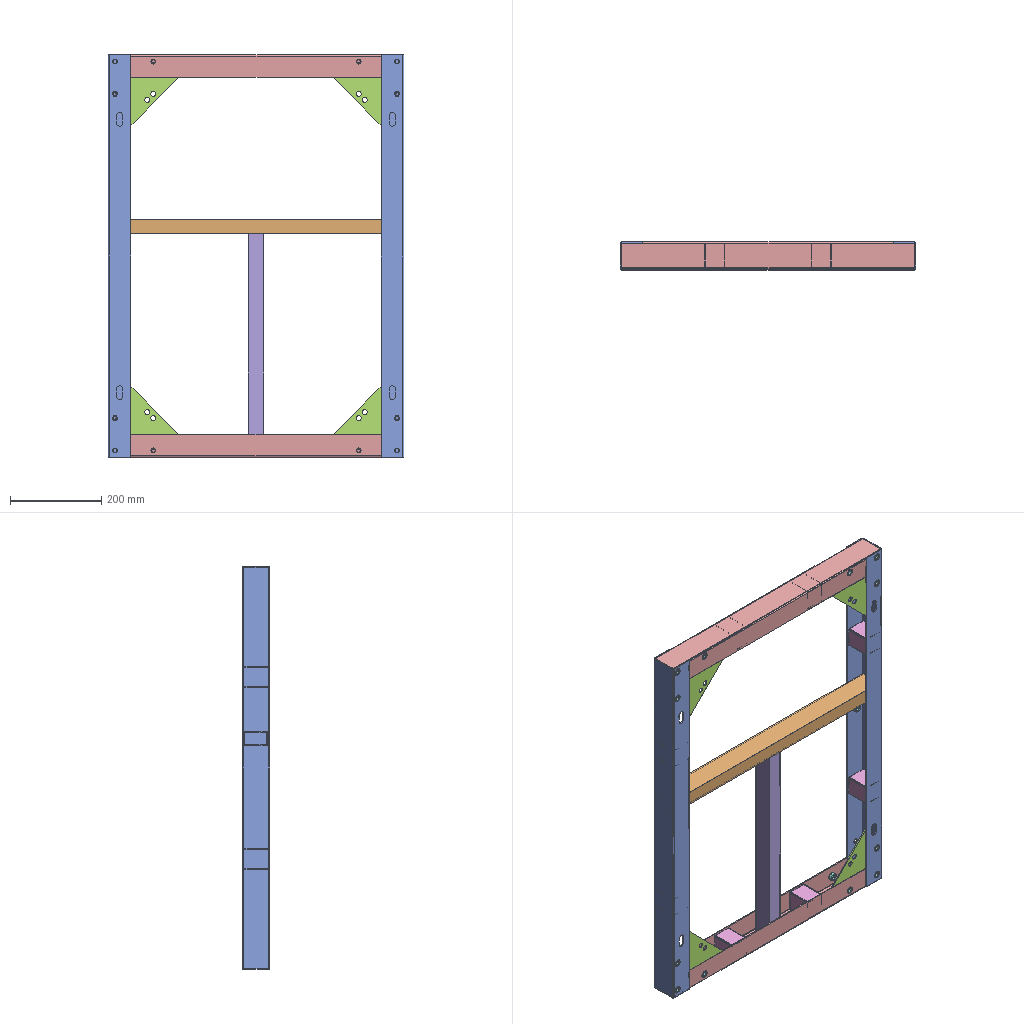Assembly | SolidWorks | 7 different items | 19 placed | box 649 x 60 x 884 mm
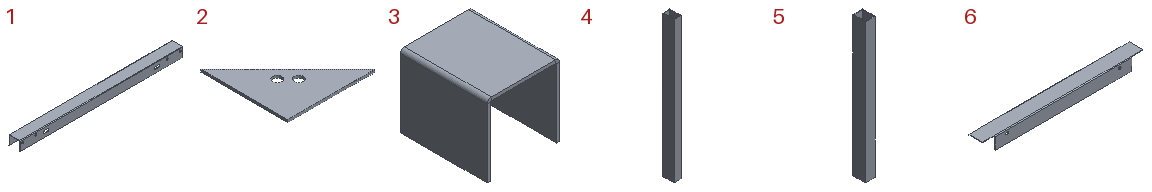Parts list (item | name | quantity | size | volume | features):
1 | - | x2 | 884 x 60 x 50 mm | 336431 mm3 | features ICE 3, Cut 2, EdgeFlange 1, FlatPattern 1, SMBaseFlange 1, SheetMetal 1
2 | - | x4 | 105 x 105 x 3 mm | 15967 mm3 | features Cut 1, FlatPattern 1, SMBaseFlange 1, SheetMetal 1
3 | - | x8 | 45 x 54 x 45 mm | 14009 mm3 | features EdgeFlange 1, FlatPattern 1, SMBaseFlange 1, SheetMetal 1
4 | - | x1 | 31.516 x 51.109 x 644 mm | 202538 mm3 | features Extrusion 1
5 | - | x1 | 35 x 44 x 488.489 mm | 146547 mm3 | features Extrusion 1
6 | - | x2 | 644 x 60 x 50 mm | 222593 mm3 | features Cut 2, EdgeFlange 1, FlatPattern 1, ICE 1, MirrorPattern 1, SMBaseFlange 1, SheetMetal 1
7 | self-clinching nut_pmm | x1 | - | - | -
Mates (type | each side: item.copy, entity, surface, feature):
Coincident | 6.1 face plane Base-Flange1 | 1.1 face plane Base-Flange1 | 2 times
Coincident | 6.1 face plane Edge-Flange1 | 1.1 face plane Edge-Flange1
Coincident | 1.1 face plane Edge-Flange1 | 2.1 face plane Base-Flange1 | 2 times
Coincident | 6.1 face plane Edge-Flange1 | 2.1 face plane Base-Flange1
Coincident | 1.1 face plane Base-Flange1 | 3.1 face plane Edge-Flange1
Coincident | 1.1 face plane Edge-Flange1 | 3.1 face plane Base-Flange1
DistanceDim | 6.1 face plane Base-Flange1 | 3.1 face plane Edge-Flange1
Coincident | 6.1 face plane Edge-Flange1 | 3.2 face plane Base-Flange1
Coincident | 6.1 face plane Base-Flange1 | 3.2 face plane Edge-Flange1
DistanceDim | 3.2 face plane Edge-Flange1 | 1.1 face plane Base-Flange1
InPlace | 1.1 face plane Base-Flange1 | assembly plane
InPlace | 6.1 face plane Base-Flange1 | assembly plane